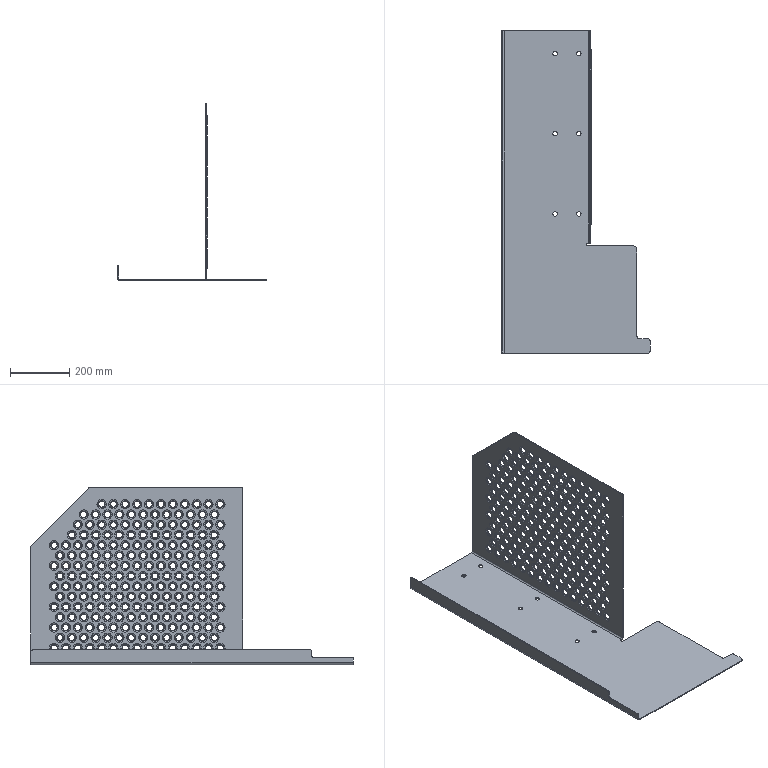Part | SolidWorks | features Fillet 2, FormToolInstance 2, ICE 2, Chamfer 1, EdgeFlange 1, FlatPattern 1, SMBaseFlange 1, SheetMetal 1 | 1 solid | 2144 faces | box 500 x 1087 x 597 mm | volume 2492497 mm3 | cone 1254 | torus 836 | cylinder 28 | plane 26 | commonest cylinder face diameters 15 x12 10 x7 20 x7 16.4 x2